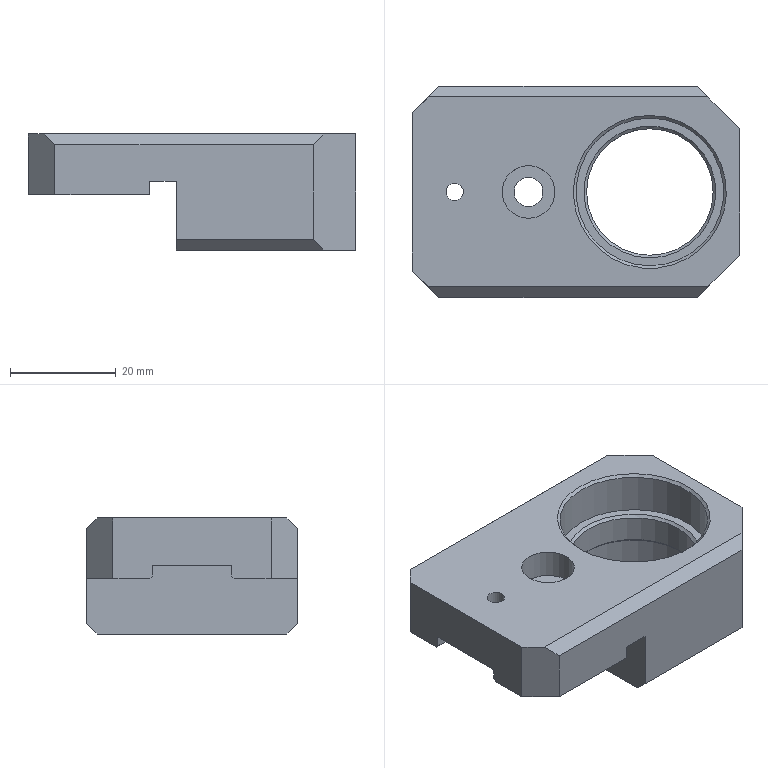NC program | NX | posted with a generic post | part box 62 x 40 x 22 mm
Whole program:
N10 G17 G21 G94 G90
(FLOOR_WALL_COPY , TOOL : D63)
N12 T01 M6
N14 G54
N16 G17 G0 G90 X-65.5 Y0. S6500 M3
N18 G43 Z30. H1
N20 Z5.
N22 G94 G1 Z2. F1500.
N24 X-62.5
N26 X62.5
N28 X65.5
N30 Z5.
N32 G0 Z30.
N34 X-65.5
N36 Z4.
N38 G1 Z1.
N40 X-62.5
N42 X62.5
N44 X65.5
N46 Z4.
N48 G0 Z30.
N50 X-65.5
N52 Z3.
N54 G1 Z0.
N56 X-62.5
N58 X62.5
N60 X65.5
N62 Z3.
N64 G0 Z30.
N66 M5
(HOLE_MILLING_COPY_1 , TOOL : D10)
N68 T04 M6
N70 G54
N72 G17 G0 G90 X-14. Y0. S7000 M3
N74 G43 Z30. H4
N76 Z0.5
N78 G94 G1 X-16.867 Y2.644 F2000.
N80 G3 X-22.9 Y0. R3.596
N82 X-22.9 Y0. Z-0.5 I8.9 J0.
N84 X-22.9 Y0. Z-1.5 I8.9 J0.
N86 X-22.9 Y0. Z-2.5 I8.9 J0.
N88 X-22.9 Y0. Z-3.5 I8.9 J0.
N90 X-22.9 Y0. Z-4.5 I8.9 J0.
N92 X-22.9 Y0. Z-5.5 I8.9 J0.
N94 X-22.9 Y0. Z-6.5 I8.9 J0.
N96 X-22.9 Y0. Z-7.5 I8.9 J0.
N98 X-5.1 Y0. Z-8. I8.9 J0.
N100 X-14. Y8.9 R8.9
N102 X-5.1 Y0. R-8.9
N104 X-11.133 Y2.644 R3.596
N106 G1 X-14. Y0.
N108 G0 Z30.
(FLOOR_WALL_1 , TOOL : D10)
N110 X37.5 Y1.
N112 Z0.555
N114 G1 Z-0.945 F1000.
N116 X37.
N118 G3 X36. Y0. R1.
N120 G1 Y-25. F3000.
N122 X8.1
N124 Y25.
N126 X36.
N128 Y0.
N130 X29.
N132 Y-18.
N134 X15.1
N136 Y18.
N138 X29.
N140 Y0.
N142 X24.5
N144 Y-13.5
N146 X19.6
N148 Y13.5
N150 X24.5
N152 Y0.
N154 G3 X25.5 Y-1. R1.
N156 G1 Z0.555
N158 G0 X37.5 Y1. Z-0.391
N160 G1 Z-1.891 F1000.
N162 X37.
N164 G3 X36. Y0. R1.
N166 G1 Y-25. F3000.
N168 X8.1
N170 Y25.
N172 X36.
N174 Y0.
N176 X29.
N178 Y-18.
N180 X15.1
N182 Y18.
N184 X29.
N186 Y0.
N188 X24.5
N190 Y-13.5
N192 X19.6
N194 Y13.5
N196 X24.5
N198 Y0.
N200 G3 X25.5 Y-1. R1.
N202 G1 Z-0.391
N204 G0 X37.5 Y1. Z-1.336
N206 G1 Z-2.836 F1000.
N208 X37.
N210 G3 X36. Y0. R1.
N212 G1 Y-25. F3000.
N214 X8.1
N216 Y25.
N218 X36.
N220 Y0.
N222 X29.
N224 Y-18.
N226 X15.1
N228 Y18.
N230 X29.
N232 Y0.
N234 X24.5
N236 Y-13.5
N238 X19.6
N240 Y13.5
N242 X24.5
N244 Y0.
N246 G3 X25.5 Y-1. R1.
N248 G1 Z-1.336
N250 G0 X37.5 Y1. Z-2.282
N252 G1 Z-3.782 F1000.
N254 X37.
N256 G3 X36. Y0. R1.
N258 G1 Y-25. F3000.
N260 X8.1
N262 Y25.
N264 X36.
N266 Y0.
N268 X29.
N270 Y-18.
N272 X15.1
N274 Y18.
N276 X29.
N278 Y0.
N280 X24.5
N282 Y-13.5
N284 X19.6
N286 Y13.5
N288 X24.5
N290 Y0.
N292 G3 X25.5 Y-1. R1.
N294 G1 Z-2.282
N296 G0 X37.5 Y1. Z-3.227
N298 G1 Z-4.727 F1000.
N300 X37.
N302 G3 X36. Y0. R1.
N304 G1 Y-25. F3000.
N306 X8.1
N308 Y25.
N310 X36.
N312 Y0.
N314 X29.
N316 Y-18.
N318 X15.1
N320 Y18.
N322 X29.
N324 Y0.
N326 X24.5
N328 Y-13.5
N330 X19.6
N332 Y13.5
N334 X24.5
N336 Y0.
N338 G3 X25.5 Y-1. R1.
N340 G1 Z-3.227
N342 G0 X37.5 Y1. Z-4.173
N344 G1 Z-5.673 F1000.
N346 X37.
N348 G3 X36. Y0. R1.
N350 G1 Y-25. F3000.
N352 X8.1
N354 Y25.
N356 X36.
N358 Y0.
N360 X29.
N362 Y-18.
N364 X15.1
N366 Y18.
N368 X29.
N370 Y0.
N372 X24.5
N374 Y-13.5
N376 X19.6
N378 Y13.5
N380 X24.5
N382 Y0.
N384 G3 X25.5 Y-1. R1.
N386 G1 Z-4.173
N388 G0 X37.5 Y1. Z-5.118
N390 G1 Z-6.618 F1000.
N392 X37.
N394 G3 X36. Y0. R1.
N396 G1 Y-25. F3000.
N398 X8.1
N400 Y25.
N402 X36.
N404 Y0.
N406 X29.
N408 Y-18.
N410 X15.1
N412 Y18.
N414 X29.
N416 Y0.
N418 X24.5
N420 Y-13.5
N422 X19.6
N424 Y13.5
N426 X24.5
N428 Y0.
N430 G3 X25.5 Y-1. R1.
N432 G1 Z-5.118
N434 G0 X37.5 Y1. Z-6.064
N436 G1 Z-7.564 F1000.
N438 X37.
N440 G3 X36. Y0. R1.
N442 G1 Y-25. F3000.
N444 X8.1
N446 Y25.
N448 X36.
N450 Y0.
N452 X29.
N454 Y-18.
N456 X15.1
N458 Y18.
N460 X29.
N462 Y0.
N464 X24.5
N466 Y-13.5
N468 X19.6
N470 Y13.5
N472 X24.5
N474 Y0.
N476 G3 X25.5 Y-1. R1.
N478 G1 Z-6.064
N480 G0 X37.5 Y1. Z-7.009
N482 G1 Z-8.509 F1000.
N484 X37.
N486 G3 X36. Y0. R1.
N488 G1 Y-25. F3000.
N490 X8.1
N492 Y25.
N494 X36.
N496 Y0.
N498 X29.
N500 Y-18.
N502 X15.1
N504 Y18.
N506 X29.
N508 Y0.
N510 X24.5
N512 Y-13.5
N514 X19.6
N516 Y13.5
N518 X24.5
N520 Y0.
N522 G3 X25.5 Y-1. R1.
N524 G1 Z-7.009
N526 G0 X37.5 Y1. Z-7.955
N528 G1 Z-9.455 F1000.
N530 X37.
N532 G3 X36. Y0. R1.
N534 G1 Y-25. F3000.
N536 X8.1
N538 Y25.
N540 X36.
N542 Y0.
N544 X29.
N546 Y-18.
N548 X15.1
N550 Y18.
N552 X29.
N554 Y0.
N556 X24.5
N558 Y-13.5
N560 X19.6
N562 Y13.5
N564 X24.5
N566 Y0.
N568 G3 X25.5 Y-1. R1.
N570 G1 Z-7.955
N572 G0 X37.5 Y1. Z-8.9
N574 G1 Z-10.4 F1000.
N576 X37.
N578 G3 X36. Y0. R1.
N580 G1 Y-25. F3000.
N582 X8.1
N584 Y25.
N586 X36.
N588 Y0.
N590 X29.
N592 Y-18.
N594 X15.1
N596 Y18.
N598 X29.
N600 Y0.
N602 X24.5
N604 Y-13.5
N606 X19.6
N608 Y13.5
N610 X24.5
N612 Y0.
N614 G3 X25.5 Y-1. R1.
N616 G1 Z-8.9
N618 G0 Z30.
(FLOOR_WALL_1_COPY , TOOL : D10)
N620 X31.997 Y26.5
N622 Z-9.
N624 G1 Z-10.5 F1000.
N626 Y26.
N628 G3 X30.997 Y25. R1.
N630 G1 Y-25. F1200.
N632 X26.498
N634 Y25.
N636 X21.998
N638 Y-25.
N640 X17.499
N642 Y25.
N644 X12.999
N646 Y-25.
N648 G3 X13.999 Y-26. R1.
N650 G1 Y-26.5
N652 Z-9.
N654 G0 Z-6.5
N656 X9. Y26.5
N658 Z-9.
N660 G1 Z-10.5 F1000.
N662 Y26.
N664 G3 X8. Y25. R1.
N666 G1 Y-25. F1200.
N668 G3 X9. Y-26. R1.
N670 G1 Y-26.5
N672 Z-9.
N674 G0 Z30.
N676 M5
(FLOOR_WALL_1_COPY_1 , TOOL : D4)
N678 T24 M6
N680 G54
N682 G17 G0 G90 X34.5 Y0.4 S7000 M3
N684 G43 Z30. H24
N686 Z-9.4
N688 G94 G1 Z-10.9 F1000.
N690 X33.4
N692 G3 X33. Y0. R0.4
N694 G1 Y-5.4 F2000.
N696 X5.9
N698 Y-22.
N700 X5.1
N702 Y22.
N704 X5.9
N706 Y5.4
N708 X33.
N710 Y0.
N712 X30.2
N714 Y-2.6
N716 X7.9
N718 Y2.6
N720 X30.2
N722 Y0.
N724 X28.4
N726 Y-0.8
N728 X9.7
N730 Y0.8
N732 X28.4
N734 Y0.
N736 G3 X28.8 Y-0.4 R0.4
N738 G1 Z-9.4
N740 G0 X34.5 Y0.4 Z-9.8
N742 G1 Z-11.3 F1000.
N744 X33.4
N746 G3 X33. Y0. R0.4
N748 G1 Y-5.4 F2000.
N750 X5.9
N752 Y-22.
N754 X5.1
N756 Y22.
N758 X5.9
N760 Y5.4
N762 X33.
N764 Y0.
N766 X30.2
N768 Y-2.6
N770 X7.9
N772 Y2.6
N774 X30.2
N776 Y0.
N778 X28.4
N780 Y-0.8
N782 X9.7
N784 Y0.8
N786 X28.4
N788 Y0.
N790 G3 X28.8 Y-0.4 R0.4
N792 G1 Z-9.8
N794 G0 X34.5 Y0.4 Z-10.2
N796 G1 Z-11.7 F1000.
N798 X33.4
N800 G3 X33. Y0. R0.4
N802 G1 Y-5.4 F2000.
N804 X5.9
N806 Y-22.
N808 X5.1
N810 Y22.
N812 X5.9
N814 Y5.4
N816 X33.
N818 Y0.
N820 X30.2
N822 Y-2.6
N824 X7.9
N826 Y2.6
N828 X30.2
N830 Y0.
N832 X28.4
N834 Y-0.8
N836 X9.7
N838 Y0.8
N840 X28.4
N842 Y0.
N844 G3 X28.8 Y-0.4 R0.4
N846 G1 Z-10.2
N848 G0 X34.5 Y0.4 Z-10.6
N850 G1 Z-12.1 F1000.
N852 X33.4
N854 G3 X33. Y0. R0.4
N856 G1 Y-5.4 F2000.
N858 X5.9
N860 Y-22.
N862 X5.1
N864 Y22.
N866 X5.9
N868 Y5.4
N870 X33.
N872 Y0.
N874 X30.2
N876 Y-2.6
N878 X7.9
N880 Y2.6
N882 X30.2
N884 Y0.
N886 X28.4
N888 Y-0.8
N890 X9.7
N892 Y0.8
N894 X28.4
N896 Y0.
N898 G3 X28.8 Y-0.4 R0.4
N900 G1 Z-10.6
N902 G0 X34.5 Y0.4 Z-11.
N904 G1 Z-12.5 F1000.
N906 X33.4
N908 G3 X33. Y0. R0.4
N910 G1 Y-5.4 F2000.
N912 X5.9
N914 Y-22.
N916 X5.1
N918 Y22.
N920 X5.9
N922 Y5.4
N924 X33.
N926 Y0.
N928 X30.2
N930 Y-2.6
N932 X7.9
N934 Y2.6
N936 X30.2
N938 Y0.
N940 X28.4
N942 Y-0.8
N944 X9.7
N946 Y0.8
N948 X28.4
N950 Y0.
N952 G3 X28.8 Y-0.4 R0.4
N954 G1 Z-11.
N956 G0 X34.5 Y0.4 Z-11.4
N958 G1 Z-12.9 F1000.
N960 X33.4
N962 G3 X33. Y0. R0.4
N964 G1 Y-5.4 F2000.
N966 X5.9
N968 Y-22.
N970 X5.1
N972 Y22.
N974 X5.9
N976 Y5.4
N978 X33.
N980 Y0.
N982 X30.2
N984 Y-2.6
N986 X7.9
N988 Y2.6
N990 X30.2
N992 Y0.
N994 X28.4
N996 Y-0.8
N998 X9.7
N1000 Y0.8
N1002 X28.4
N1004 Y0.
N1006 G3 X28.8 Y-0.4 R0.4
N1008 G1 Z-11.4
N1010 G0 Z30.
(FLOOR_WALL_1_COPY_COPY , TOOL : D4)
N1012 X34.5 Y4.9
N1014 Z-11.5
N1016 G1 Z-13. F1000.
N1018 X31.397
N1020 G3 X30.997 Y5.3 R0.4
N1022 G1 Y-5.3 F1200.
N1024 X29.013
N1026 Y5.3
N1028 X27.028
N1030 Y-5.3
N1032 X25.044
N1034 Y5.3
N1036 X23.059
N1038 Y-5.3
N1040 X21.075
N1042 Y5.3
N1044 X19.091
N1046 Y-5.3
N1048 X17.106
N1050 Y5.3
N1052 X15.122
N1054 Y-5.3
N1056 X13.138
N1058 Y5.3
N1060 X11.153
N1062 Y-5.3
N1064 X9.169
N1066 Y5.3
N1068 X7.184
N1070 Y-5.3
N1072 X6.
N1074 G3 X5.8 Y-5.5 R0.2
N1076 G1 Y-22.
N1078 X5.2
N1080 Y22.
N1082 G2 X5.6 Y22.4 R0.4
N1084 G1 Y23.5
N1086 Z-11.5
N1088 G0 Z-9.
N1090 X5.4
N1092 Z-11.5
N1094 G1 Z-13. F1000.
N1096 Y22.4
N1098 G3 X5. Y22. R0.4
N1100 G1 Y-22. F1200.
N1102 G3 X5.4 Y-22.4 R0.4
N1104 G1 X5.6
N1106 G3 X6. Y-22. R0.4 F1000.
N1108 G1 Y-5.5 F1200.
N1110 X33.
N1112 G3 X33.4 Y-5.1 R0.4
N1114 G1 X34.5
N1116 Z-11.5
N1118 G0 Z-9.
N1120 Y5.1
N1122 Z-11.5
N1124 G1 Z-13. F1000.
N1126 X33.4
N1128 G3 X33. Y5.5 R0.4
N1130 G1 X6. F1200.
N1132 Y22.
N1134 G3 X5.6 Y22.4 R0.4
N1136 G1 Y23.5
N1138 Z-11.5
N1140 G0 Z30.
N1142 M5
(PLANAR_MILL_COPY_1 , TOOL : D8A45)
N1144 T06 M6
N1146 G54
N1148 G17 G0 G90 X5.5 Y1.501 S7000 M3
N1150 G43 Z30. H6
N1152 Z0.5
N1154 G94 G1 Z-1. F1250.
N1156 X4.4 Y0.866
N1158 G3 X3.9 Y0. R1.
N1160 G1 Y-19.9
N1162 G2 X2.9 Y-20.9 R1.
N1164 G1 X-22.959
N1166 G2 X-23.666 Y-20.607 R1.
N1168 G1 X-25.636 Y-18.636
N1170 X-31.607 Y-12.666
N1172 G2 X-31.9 Y-11.959 R1.
N1174 G1 Y11.959
N1176 G2 X-31.607 Y12.666 R1.
N1178 G1 X-25.636 Y18.636
N1180 X-23.666 Y20.607
N1182 G2 X-22.959 Y20.9 R1.
N1184 G1 X2.9
N1186 G2 X3.9 Y19.9 R1.
N1188 G1 Y0.
N1190 G3 X4.4 Y-0.866 R1.
N1192 G1 X5.5 Y-1.501
N1194 Z0.5
N1196 G0 Z30.
N1198 X-2.607 Y-1.563
N1200 Z0.5
N1202 G1 Z-1.
N1204 X-1.4 Y-0.866
N1206 G3 X-0.9 Y0. R1.
N1208 X-14. Y13.1 R13.1
N1210 X-0.9 Y0. R-13.1
N1212 X-1.4 Y0.866 R1.
N1214 G1 X-2.607 Y1.563
N1216 Z0.5
N1218 G0 Z30.
(PLANAR_MILL_COPY_1_COPY , TOOL : D8A45)
N1220 X9.618 Y-5.
N1222 Z-10.
N1224 G1 Z-11.5
N1226 X8. Y-5.934
N1228 G3 X7.5 Y-6.8 R1.
N1230 G2 X8.1 Y-6.6 R1.
N1232 G1 X30.9
N1234 G2 X31.9 Y-7.6 R1.
N1236 G1 Y-14.959
N1238 G2 X31.607 Y-15.666 R1.
N1240 G1 X26.666 Y-20.607
N1242 G2 X25.959 Y-20.9 R1.
N1244 G1 X8.1
N1246 G2 X7.451 Y-20.661 R1.
N1248 G3 X7.819 Y-21.591 R1.
N1250 G1 X8.964 Y-22.5
N1252 Z-10.
N1254 G0 Z30.
N1256 Y22.5
N1258 Z-10.
N1260 G1 Z-11.5
N1262 X7.819 Y21.591
N1264 G3 X7.451 Y20.661 R1.
N1266 G2 X8.1 Y20.9 R1.
N1268 G1 X25.959
N1270 G2 X26.666 Y20.607 R1.
N1272 G1 X31.607 Y15.666
N1274 G2 X31.9 Y14.959 R1.
N1276 G1 Y7.6
N1278 G2 X30.9 Y6.6 R1.
N1280 G1 X8.1
N1282 G2 X7.5 Y6.8 R1.
N1284 G3 X8. Y5.934 R1.
N1286 G1 X9.618 Y5.
N1288 Z-10.
N1290 G0 Z30.
(PLANAR_MILL_COPY_COPY , TOOL : D8A45)
N1292 X4.501 Y-22.6
N1294 Z-1.
N1296 G1 Z-2.5
N1298 X3.866 Y-21.5
N1300 G3 X3. Y-21. R1.
N1302 G1 X-25.
N1304 G3 X-25.866 Y-21.5 R1.
N1306 G1 X-26.501 Y-22.6
N1308 Z-1.
N1310 G0 Z30.
N1312 X4.79
N1314 Z-1.
N1316 G1 Z-2.5
N1318 X3.866 Y-21.
N1320 G3 X3. Y-20.5 R1.
N1322 G1 X-25.
N1324 G3 X-25.866 Y-21. R1.
N1326 G1 X-26.79 Y-22.6
N1328 Z-1.
N1330 G0 Z30.
N1332 X-3.676 Y-1.256
N1334 Z-1.
N1336 G1 Z-2.5
N1338 X-3. Y-0.866
N1340 G3 X-2.5 Y0. R1.
N1342 X-14. Y11.5 R11.5
N1344 X-2.5 Y0. R-11.5
N1346 X-3. Y0.866 R1.
N1348 G1 X-2.5 Y-0.866
N1350 G3 X-2. Y0. R1.
N1352 X-14. Y12. R12.
N1354 X-2. Y0. R-12.
N1356 X-2.5 Y0.866 R1.
N1358 G1 X-3.719 Y1.57
N1360 Z-1.
N1362 G0 Z30.
N1364 X-26.501 Y22.6
N1366 Z-1.
N1368 G1 Z-2.5
N1370 X-25.866 Y21.5
N1372 G3 X-25. Y21. R1.
N1374 G1 X3.
N1376 G3 X3.866 Y21.5 R1.
N1378 G1 X4.501 Y22.6
N1380 Z-1.
N1382 G0 Z30.
N1384 X-26.79
N1386 Z-1.
N1388 G1 Z-2.5
N1390 X-25.866 Y21.
N1392 G3 X-25. Y20.5 R1.
N1394 G1 X3.
N1396 G3 X3.866 Y21. R1.
N1398 G1 X4.79 Y22.6
N1400 Z-1.
N1402 G0 Z30.
N1404 M5
(CUTTERCOMP4_COPY , TOOL : D10)
N1406 T04 M6
N1408 G54
N1410 G17 G0 G90 X-14. Y0. S7000 M3
N1412 G43 Z30. H4
N1414 Z0.5
N1416 G41 G94 G1 X-19.233 Y2.725 F1000. D4
N1418 G3 X-22.95 Y0. R2.857
N1420 X-22.95 Y0. Z-2.5 I8.95 J0.
N1422 X-22.95 Y0. Z-5.5 I8.95 J0.
N1424 X-18.475 Y7.751 Z-8. R-8.95
N1426 X-21.751 Y-4.475 R8.95
N1428 X-18.475 Y7.751 R-8.95
N1430 X-18.976 Y3.169 R2.857
N1432 G40
N1434 G1 X-14. Y0.
N1436 G0 Z30.
N1438 M5
N1440 M2